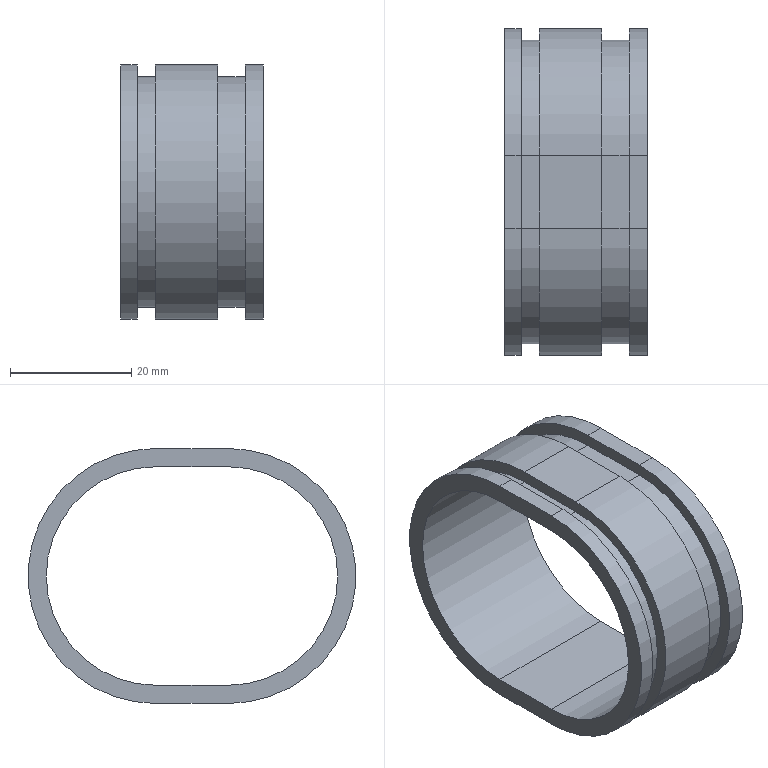Part | STEP file | 1-62 | 1 solid | 30 faces | box 23.5 x 54 x 42 mm | volume 8085 mm3 | plane 18 | cylinder 12 | commonest cylinder face diameters 42 x6 38 x4 36 x2